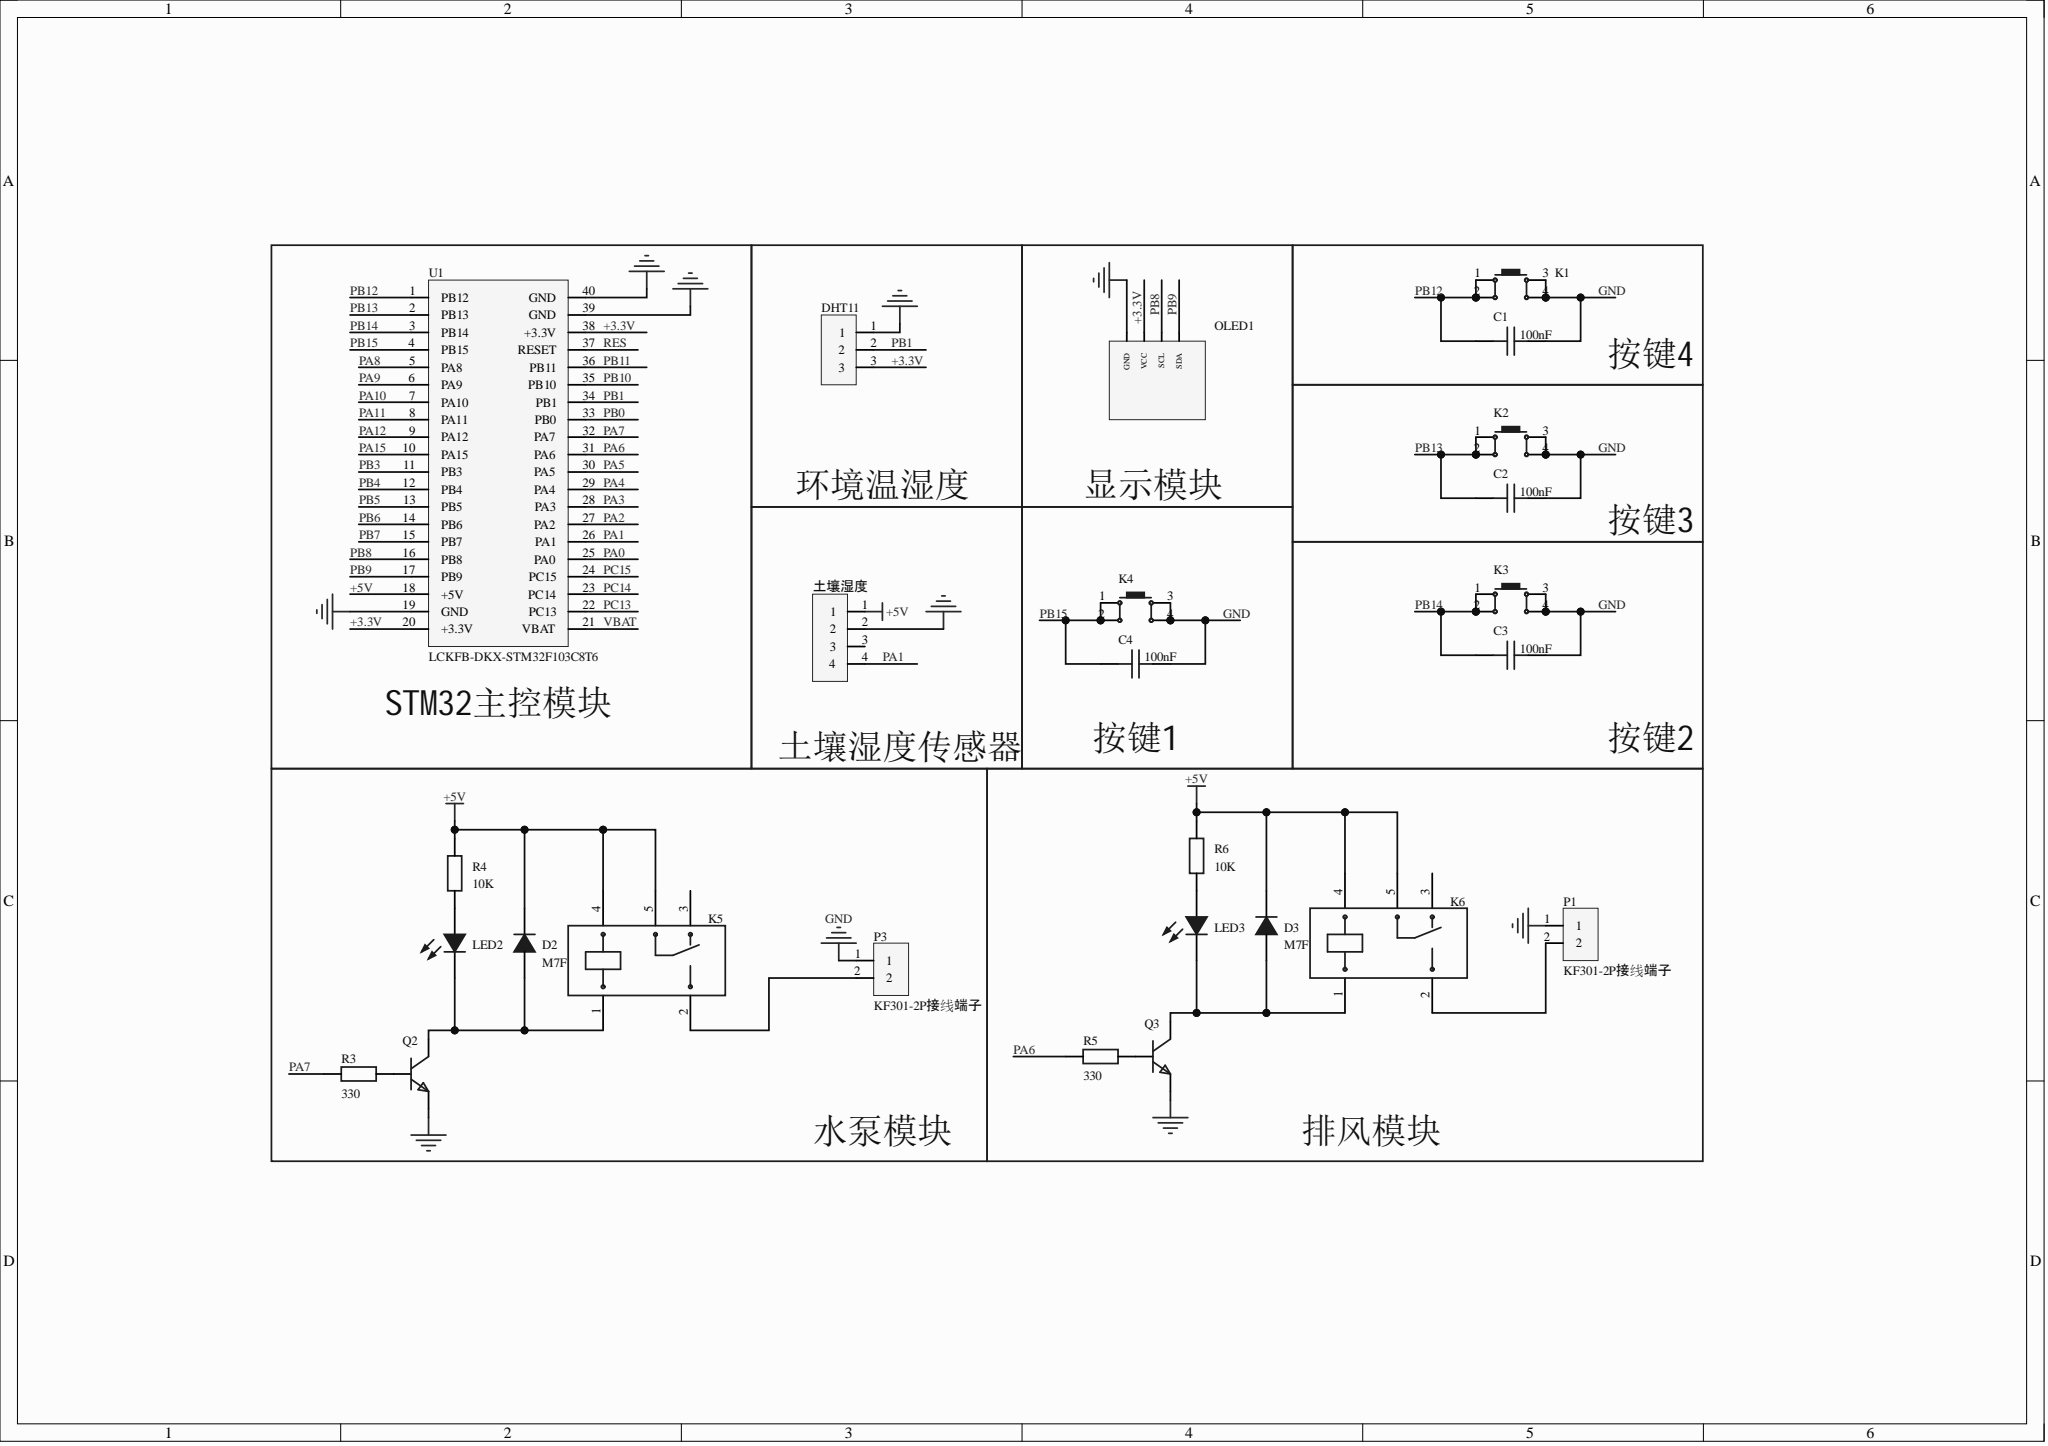Circuit board | Altium Designer | 26 parts | 21 nets
Bill of materials:
Comment,Description,Designator,Footprint,LibRef,Quantity
"100nF","容值:100nF;精度:±10%;额定电压:6.3V;材质(温度系数):X7R;","C1, C2, C3, C4","C0805","CC0603KRX7R5BB104","4"
"M7F","正向压降(Vf):1.1V@1A;直流反向耐压(Vr):1kV;整流电流:1A;","D2, D3","SMAF_L3.5-W2.6-LS4.7-RD","M7F_C22368801","2"
"","","DHT11","HDR-TH_3P-P2.54-V-M","HDR-M_2.54_1x3P","1"
"","","K1, K2, K3, K4","SW-SMD_4P-L6.0-W6.0-P4.50-LS9.0-2","Key_SMD_6x6x6.5","4"
"SRD-DC5V-SL-C","触点形式:-;","K5, K6","RELAY-TH_SRD-DCXXV-SL-C","SRD-DC5V-SL-C","2"
"MS-PTV1608NWAF-B02","","LED2, LED3","LED0805-RD_BLUE","MS-PTV1608NWAF-B02","2"
"","","OLED1","0.96OLED_4P","0.96OLED模块_4P","1"
"KF301-2P接线端子","","P1, P3","CONN-TH_XY301V-A-5.0-2P","KF301-2P接线端子","2"
"","","Q2, Q3","S8050_SOT-23","S8050_SOT_NPN","2"
"330","","R3, R5","R0805","Res_0603","2"
"10K","","R4, R6","R0805","Res_0603","2"
"LCKFB-DKX-STM32F103C8T6","","U1","CONN-TH_L53.3-W22.9_STM32F103C8T6-CARD","LCKFB-DKX-STM32F103C8T6","1"
"","","土壤湿度","HDR-TH_4P-P2.54-V-M","HDR-M_2.54_1x4P","1"
Netlist (Protel format):
[
C1
C0805
100nF



]
[
C2
C0805
100nF



]
[
C3
C0805
100nF



]
[
C4
C0805
100nF



]
[
D2
SMAF_L3.5-W2.6-LS4.7-RD
M7F



]
[
D3
SMAF_L3.5-W2.6-LS4.7-RD
M7F



]
[
DHT11
HDR-TH_3P-P2.54-V-M




]
[
K1
SW-SMD_4P-L6.0-W6.0-P4.50-LS9.0-2




]
[
K2
SW-SMD_4P-L6.0-W6.0-P4.50-LS9.0-2




]
[
K3
SW-SMD_4P-L6.0-W6.0-P4.50-LS9.0-2




]
[
K4
SW-SMD_4P-L6.0-W6.0-P4.50-LS9.0-2




]
[
K5
RELAY-TH_SRD-DCXXV-SL-C
SRD-DC5V-SL-C



]
[
K6
RELAY-TH_SRD-DCXXV-SL-C
SRD-DC5V-SL-C



]
[
LED2
LED0805-RD_BLUE
MS-PTV1608NWAF-B02



]
[
LED3
LED0805-RD_BLUE
MS-PTV1608NWAF-B02



]
[
OLED1
0.96OLED_4P




]
[
P1
CONN-TH_XY301V-A-5.0-2P
KF301-2P接线端子



]
[
P3
CONN-TH_XY301V-A-5.0-2P
KF301-2P接线端子



]
[
Q2
S8050_SOT-23




]
[
Q3
S8050_SOT-23




]
[
R3
R0805
330



]
[
R4
R0805
10K



]
[
R5
R0805
330



]
[
R6
R0805
10K



]
[
U1
CONN-TH_L53.3-W22.9_STM32F103C8T6-CARD
LCKFB-DKX-STM32F103C8T6



]
[
土壤湿度
HDR-TH_4P-P2.54-V-M




]
(
PB15
C4-1
K4-1
K4-2
U1-4
)
(
PB14
C3-1
K3-1
K3-2
U1-3
)
(
PB13
C2-1
K2-1
K2-2
U1-2
)
(
PB12
C1-1
K1-1
K1-2
U1-1
)
(
PB9
OLED1-4
U1-17
)
(
PB8
OLED1-3
U1-16
)
(
PB1
DHT11-2
U1-34
)
(
PA7
R3-2
U1-32
)
(
PA6
R5-2
U1-31
)
(
PA1
U1-26
土壤湿度-4
)
(
NetQ3_1
Q3-1
R5-1
)
(
NetQ2_1
Q2-1
R3-1
)
(
NetLED3_2
LED3-2
R6-1
)
(
NetLED2_2
LED2-2
R4-1
)
(
NetK6_2
K6-2
P1-2
)
(
NetK5_2
K5-2
P3-2
)
(
NetD3_2
D3-2
K6-1
LED3-1
Q3-3
)
(
NetD2_2
D2-2
K5-1
LED2-1
Q2-3
)
(
GND
C1-2
C2-2
C3-2
C4-2
DHT11-1
K1-3
K1-4
K2-3
K2-4
K3-3
K3-4
K4-3
K4-4
OLED1-1
P1-1
P3-1
Q2-2
Q3-2
U1-19
U1-39
U1-40
土壤湿度-2
)
(
+5V
D2-1
D3-1
K5-4
K5-5
K6-4
K6-5
R4-2
R6-2
U1-18
土壤湿度-1
)
(
+3.3V
DHT11-3
OLED1-2
U1-20
U1-38
)